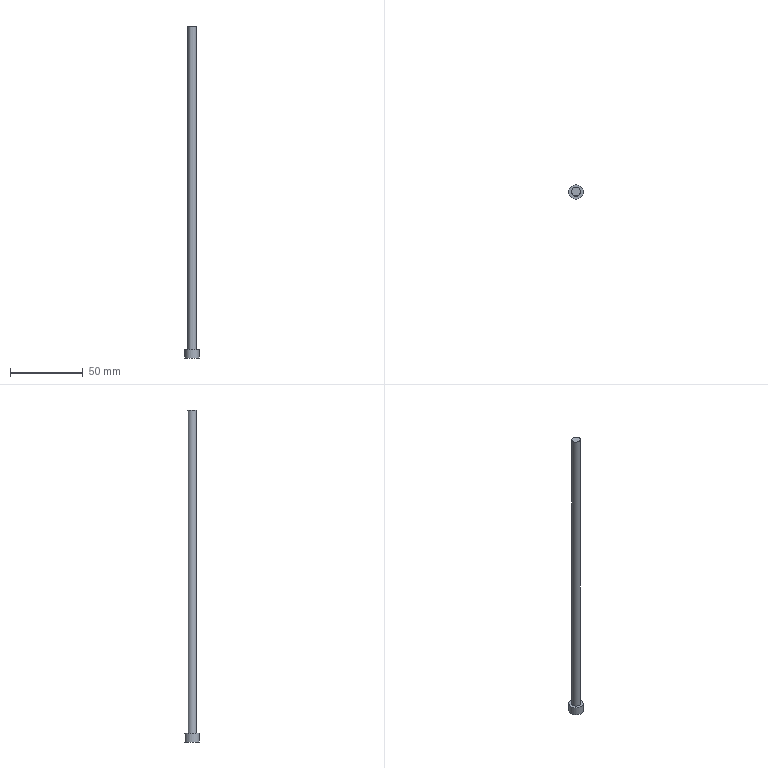Part | NX | features DDZ6.00 2 | 1 solid | 5 faces | box 10 x 10 x 228.27 mm | volume 6756 mm3 | plane 3 | cylinder 2 | commonest cylinder face diameters 6 x1 10 x1
STEP:
#1=CARTESIAN_POINT('',(7.98,-5.66,17.77));
#2=VERTEX_POINT('',#1);
#3=CARTESIAN_POINT('',(10.98,-5.66,17.77));
#4=DIRECTION('',(0.,0.,-1.));
#5=DIRECTION('',(-1.,0.,0.));
#6=AXIS2_PLACEMENT_3D('',#3,#4,#5);
#7=CIRCLE('',#6,3.);
#8=EDGE_CURVE('',#2,#2,#7,.F.);
#9=ORIENTED_EDGE('',*,*,#8,.F.);
#10=EDGE_LOOP('',(#9));
#11=FACE_BOUND('',#10,.T.);
#12=CARTESIAN_POINT('',(13.98,-5.66,-204.5));
#13=VERTEX_POINT('',#12);
#14=CARTESIAN_POINT('',(10.98,-5.66,-204.5));
#15=DIRECTION('',(0.,0.,1.));
#16=DIRECTION('',(1.,0.,0.));
#17=AXIS2_PLACEMENT_3D('',#14,#15,#16);
#18=CIRCLE('',#17,3.);
#19=EDGE_CURVE('',#13,#13,#18,.F.);
#20=ORIENTED_EDGE('',*,*,#19,.F.);
#21=EDGE_LOOP('',(#20));
#22=FACE_BOUND('',#21,.T.);
#23=CARTESIAN_POINT('',(10.98,-5.66,-210.5));
#24=DIRECTION('',(0.,0.,1.));
#25=DIRECTION('',(1.,0.,0.));
#26=AXIS2_PLACEMENT_3D('',#23,#24,#25);
#27=CYLINDRICAL_SURFACE('',#26,3.);
#28=ADVANCED_FACE('',(#11,#22),#27,.T.);
#29=ORIENTED_EDGE('',*,*,#19,.T.);
#30=EDGE_LOOP('',(#29));
#31=FACE_BOUND('',#30,.T.);
#32=CARTESIAN_POINT('',(15.98,-5.66,-204.5));
#33=VERTEX_POINT('',#32);
#34=CARTESIAN_POINT('',(10.98,-5.66,-204.5));
#35=DIRECTION('',(0.,0.,-1.));
#36=DIRECTION('',(1.,0.,0.));
#37=AXIS2_PLACEMENT_3D('',#34,#35,#36);
#38=CIRCLE('',#37,5.);
#39=EDGE_CURVE('',#33,#33,#38,.T.);
#40=ORIENTED_EDGE('',*,*,#39,.F.);
#41=EDGE_LOOP('',(#40));
#42=FACE_BOUND('',#41,.T.);
#43=CARTESIAN_POINT('',(10.98,-5.66,-204.5));
#44=DIRECTION('',(0.,0.,1.));
#45=DIRECTION('',(1.,0.,0.));
#46=AXIS2_PLACEMENT_3D('',#43,#44,#45);
#47=PLANE('',#46);
#48=ADVANCED_FACE('',(#31,#42),#47,.T.);
#49=ORIENTED_EDGE('',*,*,#39,.T.);
#50=EDGE_LOOP('',(#49));
#51=FACE_BOUND('',#50,.T.);
#52=CARTESIAN_POINT('',(15.98,-5.66,-210.5));
#53=VERTEX_POINT('',#52);
#54=CARTESIAN_POINT('',(10.98,-5.66,-210.5));
#55=DIRECTION('',(0.,0.,1.));
#56=DIRECTION('',(1.,0.,0.));
#57=AXIS2_PLACEMENT_3D('',#54,#55,#56);
#58=CIRCLE('',#57,5.);
#59=EDGE_CURVE('',#53,#53,#58,.T.);
#60=ORIENTED_EDGE('',*,*,#59,.T.);
#61=EDGE_LOOP('',(#60));
#62=FACE_BOUND('',#61,.T.);
#63=CARTESIAN_POINT('',(10.98,-5.66,-210.5));
#64=DIRECTION('',(0.,0.,1.));
#65=DIRECTION('',(1.,0.,0.));
#66=AXIS2_PLACEMENT_3D('',#63,#64,#65);
#67=CYLINDRICAL_SURFACE('',#66,5.);
#68=ADVANCED_FACE('',(#51,#62),#67,.T.);
#69=ORIENTED_EDGE('',*,*,#59,.F.);
#70=EDGE_LOOP('',(#69));
#71=FACE_BOUND('',#70,.T.);
#72=CARTESIAN_POINT('',(10.98,-5.66,-210.5));
#73=DIRECTION('',(0.,0.,-1.));
#74=DIRECTION('',(-1.,0.,0.));
#75=AXIS2_PLACEMENT_3D('',#72,#73,#74);
#76=PLANE('',#75);
#77=ADVANCED_FACE('',(#71),#76,.T.);
#78=ORIENTED_EDGE('',*,*,#8,.T.);
#79=EDGE_LOOP('',(#78));
#80=FACE_BOUND('',#79,.T.);
#81=CARTESIAN_POINT('',(0.,0.,17.77));
#82=DIRECTION('',(0.,0.,-1.));
#83=DIRECTION('',(1.,0.,0.));
#84=AXIS2_PLACEMENT_3D('',#81,#82,#83);
#85=PLANE('',#84);
#86=ADVANCED_FACE('',(#80),#85,.F.);
#87=CLOSED_SHELL('',(#28,#48,#68,#77,#86));
#88=MANIFOLD_SOLID_BREP('',#87);
#89=(LENGTH_UNIT()NAMED_UNIT(*)SI_UNIT(.MILLI.,.METRE.));
#90=UNCERTAINTY_MEASURE_WITH_UNIT(LENGTH_MEASURE(0.00001),#89,'','');
#91=(NAMED_UNIT(*)PLANE_ANGLE_UNIT()SI_UNIT($,.RADIAN.));
#92=(NAMED_UNIT(*)SI_UNIT($,.STERADIAN.)SOLID_ANGLE_UNIT());
#93=(GEOMETRIC_REPRESENTATION_CONTEXT(3)GLOBAL_UNCERTAINTY_ASSIGNED_CONTEXT((#90))GLOBAL_UNIT_ASSIGNED_CONTEXT((#89,#91,#92))REPRESENTATION_CONTEXT('',''));
#94=ADVANCED_BREP_SHAPE_REPRESENTATION('',(#88),#93);